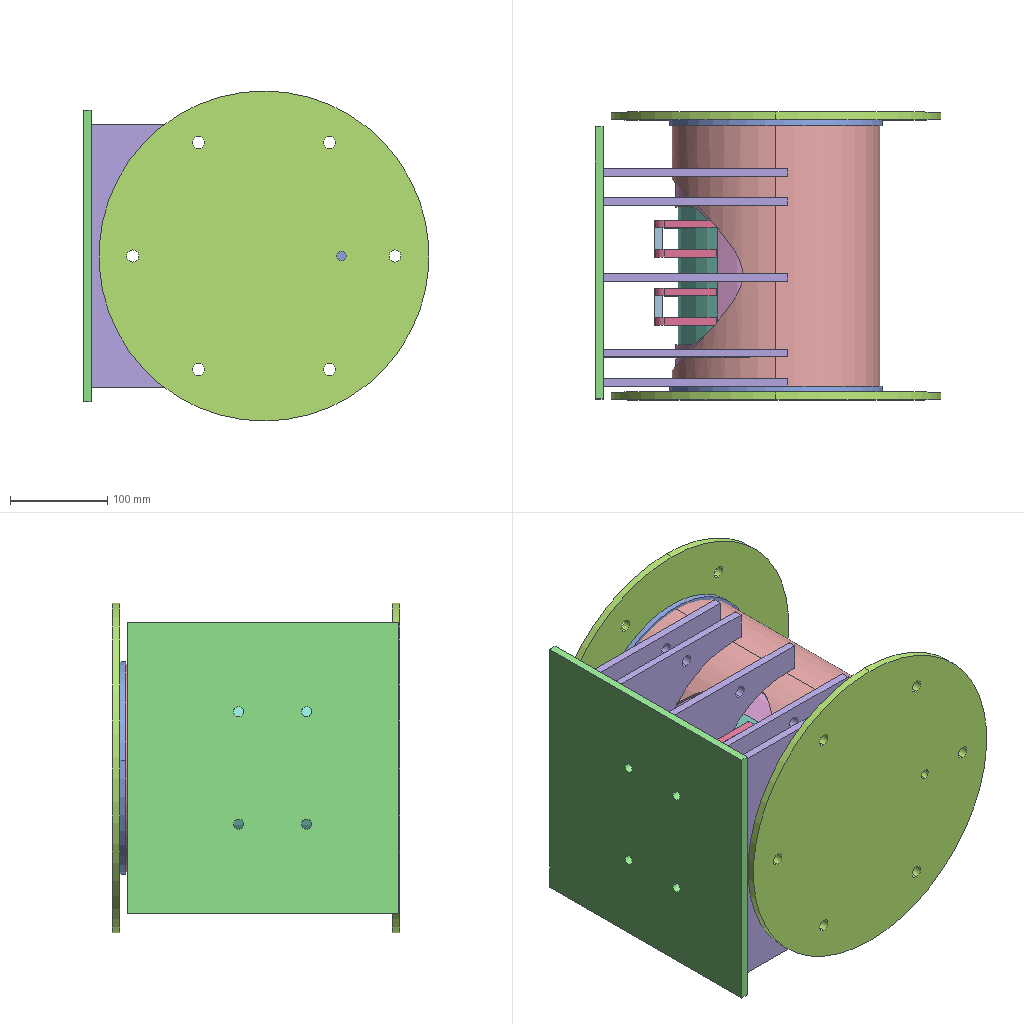Assembly | SolidWorks | 10 different items | 24 placed | box 356 x 296 x 340 mm
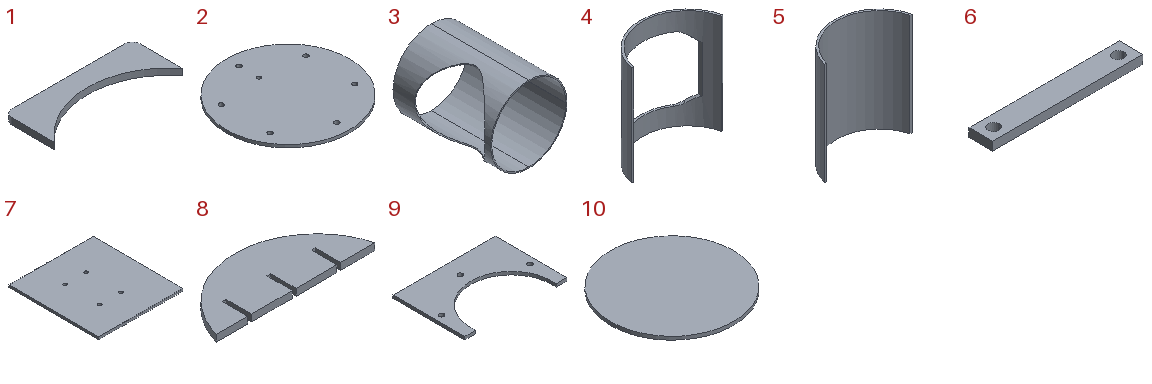Parts list (item | quantity | size | volume | features):
1 | x4 | 160 x 63.348 x 8 mm | 45593 mm3 | features Extrusion 1, Fillet 1
2 | x2 | 340 x 340 x 8 mm | 719786 mm3 | features ICE 2, Extrusion 1
3 | x1 | 213.699 x 273 x 213.7 mm | 459194 mm3 | features BaseBody 1
4 | x1 | 202.195 x 81.782 x 220 mm | 150063 mm3 | features FlatPattern 1, ICE 1, SMBaseFlange 1, SheetMetal 1
5 | x1 | 195.714 x 76 x 230 mm | 268771 mm3 | features FlatPattern 1, ICE 1, SMBaseFlange 1, SheetMetal 1
6 | x2 | 140 x 22 x 8 mm | 23255 mm3 | features Extrusion 1, ICE 1
7 | x1 | 280 x 300 x 8 mm | 669229 mm3 | features Extrusion 1, ICE 1
8 | x5 | 186.411 x 71.5 x 8 mm | 75617 mm3 | features ICE 2, Extrusion 1
9 | x5 | 270 x 190 x 8 mm | 243470 mm3 | features Cut 1, Extrusion 1
10 | x2 | 220 x 220 x 6 mm | 228080 mm3 | features Extrusion 1
Mates (type | each side: item.copy, entity, surface, feature):
Coincident | 3.1 face plane Input1 | 10.1 face plane Boss-Extrude1
Concentric | 3.1 face cylinder Input1 | 10.1 face cylinder Boss-Extrude1
Coincident | 10.1 face plane Boss-Extrude1 | 2.1 face plane Boss-Extrude1
Concentric | 10.1 face cylinder Boss-Extrude1 | 2.1 face cylinder Boss-Extrude1
Parallel | 10.2 face plane Boss-Extrude1 | 4.1 face plane Base Bend1
Parallel | 2.2 face plane Boss-Extrude1 | 5.1 face plane Base Bend1
Parallel | 2.2 face plane Boss-Extrude1 | 8.1 face plane Boss-Extrude1
Concentric | 5.1 face cylinder Base Bend1 | 8.1 face cylinder Boss-Extrude1
Concentric | 3.1 face cylinder Input1 | 9.1 face cylinder Boss-Extrude1
Parallel | 3.1 plane | 9.2 face plane Boss-Extrude1
Parallel | 3.1 face plane Input1 | 2.2 face plane Boss-Extrude1
Coincident | 9.2 face plane Boss-Extrude1 | 7.1 face plane Boss-Extrude1
Concentric | 5.1 face cylinder Base Bend1 | 1.1 face cylinder Boss-Extrude1
DistanceDim | 9.3 face plane Boss-Extrude1 | 1.1 face plane Boss-Extrude1
Coincident | 1.2 face plane Boss-Extrude1 | 6.1 face plane Boss-Extrude1
Parallel | 1.1 face plane Boss-Extrude1 | 6.1 face plane Boss-Extrude1
Coincident | 1.1 edge | 6.1 vertex
Coincident | 3.1 face plane Input1 | 5.1 face plane Base Bend1
Concentric | 7.1 face cylinder Cut-Extrude1 | 6.1 face cylinder Cut-Extrude1
Concentric | 7.1 face cylinder Cut-Extrude1 | 6.2 face cylinder Cut-Extrude1
Coincident | 5.1 face plane Cut-Extrude1 | 8.2 face plane Cut-Extrude1